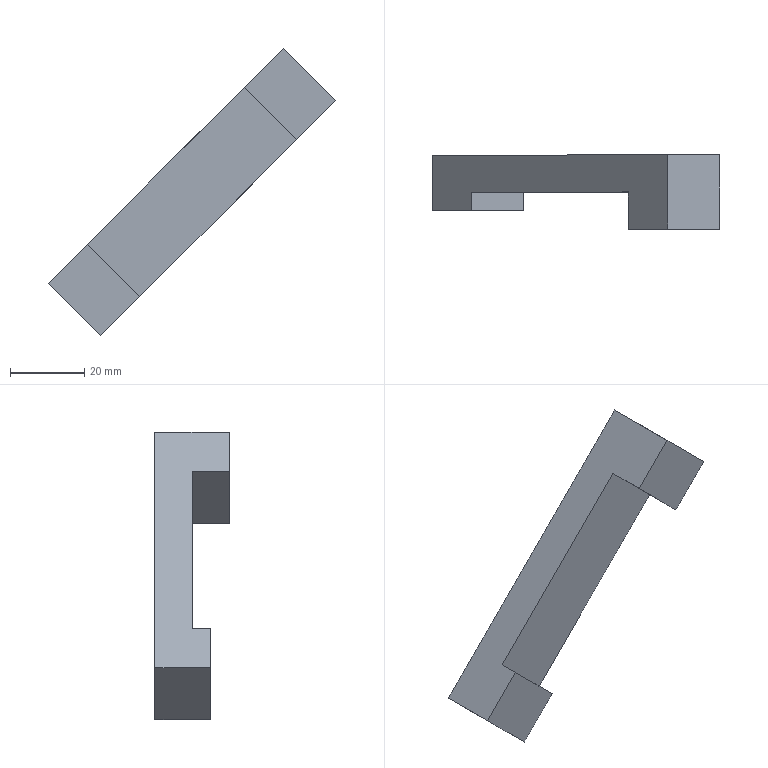Part | NX | features solid 2 | 1 solid | 10 faces | box 77.441 x 20 x 77.441 mm | volume 22280 mm3 | plane 10
STEP:
#1=CARTESIAN_POINT('',(973.987,320.,-96.61));
#2=VERTEX_POINT('',#1);
#3=CARTESIAN_POINT('',(988.034,320.,-110.657));
#4=VERTEX_POINT('',#3);
#5=CARTESIAN_POINT('',(975.003,320.,-97.625));
#6=DIRECTION('',(0.7071,0.,-0.7071));
#7=VECTOR('',#6,1000.);
#8=LINE('',#5,#7);
#9=EDGE_CURVE('',#2,#4,#8,.T.);
#10=ORIENTED_EDGE('',*,*,#9,.T.);
#11=CARTESIAN_POINT('',(1030.215,320.,-68.476));
#12=VERTEX_POINT('',#11);
#13=CARTESIAN_POINT('',(1044.239,320.,-54.452));
#14=DIRECTION('',(0.7071,0.,0.7071));
#15=VECTOR('',#14,1000.);
#16=LINE('',#13,#15);
#17=EDGE_CURVE('',#12,#4,#16,.F.);
#18=ORIENTED_EDGE('',*,*,#17,.F.);
#19=CARTESIAN_POINT('',(1016.168,320.,-54.429));
#20=VERTEX_POINT('',#19);
#21=CARTESIAN_POINT('',(1017.184,320.,-55.445));
#22=DIRECTION('',(-0.7071,0.,0.7071));
#23=VECTOR('',#22,1000.);
#24=LINE('',#21,#23);
#25=EDGE_CURVE('',#12,#20,#24,.T.);
#26=ORIENTED_EDGE('',*,*,#25,.T.);
#27=CARTESIAN_POINT('',(1023.864,320.,-46.733));
#28=DIRECTION('',(-0.7071,0.,-0.7071));
#29=VECTOR('',#28,1000.);
#30=LINE('',#27,#29);
#31=EDGE_CURVE('',#20,#2,#30,.T.);
#32=ORIENTED_EDGE('',*,*,#31,.T.);
#33=EDGE_LOOP('',(#10,#18,#26,#32));
#34=FACE_BOUND('',#33,.T.);
#35=CARTESIAN_POINT('',(1031.207,320.,-41.421));
#36=DIRECTION('',(0.,1.,0.));
#37=DIRECTION('',(-0.9796,0.,0.2008));
#38=AXIS2_PLACEMENT_3D('',#35,#36,#37);
#39=PLANE('',#38);
#40=ADVANCED_FACE('',(#34),#39,.F.);
#41=CARTESIAN_POINT('',(988.034,315.,-110.657));
#42=VERTEX_POINT('',#41);
#43=CARTESIAN_POINT('',(988.034,320.,-110.657));
#44=DIRECTION('',(0.,-1.,0.));
#45=VECTOR('',#44,1000.);
#46=LINE('',#43,#45);
#47=EDGE_CURVE('',#42,#4,#46,.F.);
#48=ORIENTED_EDGE('',*,*,#47,.F.);
#49=CARTESIAN_POINT('',(977.428,315.,-121.263));
#50=VERTEX_POINT('',#49);
#51=CARTESIAN_POINT('',(980.599,315.,-118.092));
#52=DIRECTION('',(-0.7071,0.,-0.7071));
#53=VECTOR('',#52,1000.);
#54=LINE('',#51,#53);
#55=EDGE_CURVE('',#50,#42,#54,.F.);
#56=ORIENTED_EDGE('',*,*,#55,.F.);
#57=CARTESIAN_POINT('',(977.428,330.,-121.263));
#58=VERTEX_POINT('',#57);
#59=CARTESIAN_POINT('',(977.428,320.,-121.263));
#60=DIRECTION('',(0.,-1.,0.));
#61=VECTOR('',#60,1000.);
#62=LINE('',#59,#61);
#63=EDGE_CURVE('',#50,#58,#62,.F.);
#64=ORIENTED_EDGE('',*,*,#63,.T.);
#65=CARTESIAN_POINT('',(1040.822,330.,-57.869));
#66=VERTEX_POINT('',#65);
#67=CARTESIAN_POINT('',(1044.239,330.,-54.452));
#68=DIRECTION('',(0.7071,0.,0.7071));
#69=VECTOR('',#68,1000.);
#70=LINE('',#67,#69);
#71=EDGE_CURVE('',#66,#58,#70,.F.);
#72=ORIENTED_EDGE('',*,*,#71,.F.);
#73=CARTESIAN_POINT('',(1040.822,310.,-57.869));
#74=VERTEX_POINT('',#73);
#75=CARTESIAN_POINT('',(1040.822,320.,-57.869));
#76=DIRECTION('',(0.,1.,0.));
#77=VECTOR('',#76,1000.);
#78=LINE('',#75,#77);
#79=EDGE_CURVE('',#66,#74,#78,.F.);
#80=ORIENTED_EDGE('',*,*,#79,.T.);
#81=CARTESIAN_POINT('',(1030.215,310.,-68.476));
#82=VERTEX_POINT('',#81);
#83=CARTESIAN_POINT('',(1044.239,310.,-54.452));
#84=DIRECTION('',(0.7071,0.,0.7071));
#85=VECTOR('',#84,1000.);
#86=LINE('',#83,#85);
#87=EDGE_CURVE('',#74,#82,#86,.F.);
#88=ORIENTED_EDGE('',*,*,#87,.T.);
#89=CARTESIAN_POINT('',(1030.215,320.,-68.476));
#90=DIRECTION('',(0.,1.,0.));
#91=VECTOR('',#90,1000.);
#92=LINE('',#89,#91);
#93=EDGE_CURVE('',#12,#82,#92,.F.);
#94=ORIENTED_EDGE('',*,*,#93,.F.);
#95=ORIENTED_EDGE('',*,*,#17,.T.);
#96=EDGE_LOOP('',(#48,#56,#64,#72,#80,#88,#94,#95));
#97=FACE_BOUND('',#96,.T.);
#98=CARTESIAN_POINT('',(1036.273,320.,-62.418));
#99=DIRECTION('',(0.7071,0.,-0.7071));
#100=DIRECTION('',(-0.7071,0.,-0.7071));
#101=AXIS2_PLACEMENT_3D('',#98,#99,#100);
#102=PLANE('',#101);
#103=ADVANCED_FACE('',(#97),#102,.T.);
#104=CARTESIAN_POINT('',(963.381,330.,-107.216));
#105=VERTEX_POINT('',#104);
#106=CARTESIAN_POINT('',(963.381,315.,-107.216));
#107=VERTEX_POINT('',#106);
#108=CARTESIAN_POINT('',(963.381,320.,-107.216));
#109=DIRECTION('',(0.,-1.,0.));
#110=VECTOR('',#109,1000.);
#111=LINE('',#108,#110);
#112=EDGE_CURVE('',#105,#107,#111,.T.);
#113=ORIENTED_EDGE('',*,*,#112,.T.);
#114=CARTESIAN_POINT('',(973.987,315.,-96.61));
#115=VERTEX_POINT('',#114);
#116=CARTESIAN_POINT('',(1023.864,315.,-46.733));
#117=DIRECTION('',(0.7071,0.,0.7071));
#118=VECTOR('',#117,1000.);
#119=LINE('',#116,#118);
#120=EDGE_CURVE('',#107,#115,#119,.T.);
#121=ORIENTED_EDGE('',*,*,#120,.T.);
#122=CARTESIAN_POINT('',(973.987,320.,-96.61));
#123=DIRECTION('',(0.,-1.,0.));
#124=VECTOR('',#123,1000.);
#125=LINE('',#122,#124);
#126=EDGE_CURVE('',#2,#115,#125,.T.);
#127=ORIENTED_EDGE('',*,*,#126,.F.);
#128=ORIENTED_EDGE('',*,*,#31,.F.);
#129=CARTESIAN_POINT('',(1016.168,310.,-54.429));
#130=VERTEX_POINT('',#129);
#131=CARTESIAN_POINT('',(1016.168,320.,-54.429));
#132=DIRECTION('',(0.,1.,0.));
#133=VECTOR('',#132,1000.);
#134=LINE('',#131,#133);
#135=EDGE_CURVE('',#130,#20,#134,.T.);
#136=ORIENTED_EDGE('',*,*,#135,.F.);
#137=CARTESIAN_POINT('',(1026.775,310.,-43.822));
#138=VERTEX_POINT('',#137);
#139=CARTESIAN_POINT('',(1023.864,310.,-46.733));
#140=DIRECTION('',(-0.7071,0.,-0.7071));
#141=VECTOR('',#140,1000.);
#142=LINE('',#139,#141);
#143=EDGE_CURVE('',#138,#130,#142,.T.);
#144=ORIENTED_EDGE('',*,*,#143,.F.);
#145=CARTESIAN_POINT('',(1026.775,330.,-43.822));
#146=VERTEX_POINT('',#145);
#147=CARTESIAN_POINT('',(1026.775,320.,-43.822));
#148=DIRECTION('',(0.,1.,0.));
#149=VECTOR('',#148,1000.);
#150=LINE('',#147,#149);
#151=EDGE_CURVE('',#138,#146,#150,.T.);
#152=ORIENTED_EDGE('',*,*,#151,.T.);
#153=CARTESIAN_POINT('',(1023.864,330.,-46.733));
#154=DIRECTION('',(-0.7071,0.,-0.7071));
#155=VECTOR('',#154,1000.);
#156=LINE('',#153,#155);
#157=EDGE_CURVE('',#146,#105,#156,.T.);
#158=ORIENTED_EDGE('',*,*,#157,.T.);
#159=EDGE_LOOP('',(#113,#121,#127,#128,#136,#144,#152,#158));
#160=FACE_BOUND('',#159,.T.);
#161=CARTESIAN_POINT('',(1023.864,320.,-46.733));
#162=DIRECTION('',(0.7071,0.,-0.7071));
#163=DIRECTION('',(-0.7071,0.,-0.7071));
#164=AXIS2_PLACEMENT_3D('',#161,#162,#163);
#165=PLANE('',#164);
#166=ADVANCED_FACE('',(#160),#165,.F.);
#167=CARTESIAN_POINT('',(964.397,330.,-108.232));
#168=DIRECTION('',(0.7071,0.,-0.7071));
#169=VECTOR('',#168,1000.);
#170=LINE('',#167,#169);
#171=EDGE_CURVE('',#105,#58,#170,.T.);
#172=ORIENTED_EDGE('',*,*,#171,.F.);
#173=ORIENTED_EDGE('',*,*,#157,.F.);
#174=CARTESIAN_POINT('',(1027.79,330.,-44.838));
#175=DIRECTION('',(-0.7071,0.,0.7071));
#176=VECTOR('',#175,1000.);
#177=LINE('',#174,#176);
#178=EDGE_CURVE('',#66,#146,#177,.T.);
#179=ORIENTED_EDGE('',*,*,#178,.F.);
#180=ORIENTED_EDGE('',*,*,#71,.T.);
#181=EDGE_LOOP('',(#172,#173,#179,#180));
#182=FACE_BOUND('',#181,.T.);
#183=CARTESIAN_POINT('',(1031.207,330.,-41.421));
#184=DIRECTION('',(0.,1.,0.));
#185=DIRECTION('',(-0.9796,0.,0.2008));
#186=AXIS2_PLACEMENT_3D('',#183,#184,#185);
#187=PLANE('',#186);
#188=ADVANCED_FACE('',(#182),#187,.T.);
#189=CARTESIAN_POINT('',(1027.79,310.,-44.838));
#190=DIRECTION('',(-0.7071,0.,0.7071));
#191=VECTOR('',#190,1000.);
#192=LINE('',#189,#191);
#193=EDGE_CURVE('',#74,#138,#192,.T.);
#194=ORIENTED_EDGE('',*,*,#193,.T.);
#195=ORIENTED_EDGE('',*,*,#143,.T.);
#196=CARTESIAN_POINT('',(1017.184,310.,-55.445));
#197=DIRECTION('',(-0.7071,0.,0.7071));
#198=VECTOR('',#197,1000.);
#199=LINE('',#196,#198);
#200=EDGE_CURVE('',#82,#130,#199,.T.);
#201=ORIENTED_EDGE('',*,*,#200,.F.);
#202=ORIENTED_EDGE('',*,*,#87,.F.);
#203=EDGE_LOOP('',(#194,#195,#201,#202));
#204=FACE_BOUND('',#203,.T.);
#205=CARTESIAN_POINT('',(1031.207,310.,-41.421));
#206=DIRECTION('',(0.,1.,0.));
#207=DIRECTION('',(-0.9796,0.,0.2008));
#208=AXIS2_PLACEMENT_3D('',#205,#206,#207);
#209=PLANE('',#208);
#210=ADVANCED_FACE('',(#204),#209,.F.);
#211=ORIENTED_EDGE('',*,*,#55,.T.);
#212=CARTESIAN_POINT('',(975.003,315.,-97.625));
#213=DIRECTION('',(-0.7071,0.,0.7071));
#214=VECTOR('',#213,1000.);
#215=LINE('',#212,#214);
#216=EDGE_CURVE('',#42,#115,#215,.T.);
#217=ORIENTED_EDGE('',*,*,#216,.T.);
#218=ORIENTED_EDGE('',*,*,#120,.F.);
#219=CARTESIAN_POINT('',(964.397,315.,-108.232));
#220=DIRECTION('',(-0.7071,0.,0.7071));
#221=VECTOR('',#220,1000.);
#222=LINE('',#219,#221);
#223=EDGE_CURVE('',#50,#107,#222,.T.);
#224=ORIENTED_EDGE('',*,*,#223,.F.);
#225=EDGE_LOOP('',(#211,#217,#218,#224));
#226=FACE_BOUND('',#225,.T.);
#227=CARTESIAN_POINT('',(967.568,315.,-105.06));
#228=DIRECTION('',(0.,-1.,0.));
#229=DIRECTION('',(0.9796,0.,-0.2008));
#230=AXIS2_PLACEMENT_3D('',#227,#228,#229);
#231=PLANE('',#230);
#232=ADVANCED_FACE('',(#226),#231,.T.);
#233=ORIENTED_EDGE('',*,*,#171,.T.);
#234=ORIENTED_EDGE('',*,*,#63,.F.);
#235=ORIENTED_EDGE('',*,*,#223,.T.);
#236=ORIENTED_EDGE('',*,*,#112,.F.);
#237=EDGE_LOOP('',(#233,#234,#235,#236));
#238=FACE_BOUND('',#237,.T.);
#239=CARTESIAN_POINT('',(993.082,180.,-136.918));
#240=DIRECTION('',(-0.7071,0.,-0.7071));
#241=DIRECTION('',(0.7071,0.,-0.7071));
#242=AXIS2_PLACEMENT_3D('',#239,#240,#241);
#243=PLANE('',#242);
#244=ADVANCED_FACE('',(#238),#243,.T.);
#245=ORIENTED_EDGE('',*,*,#178,.T.);
#246=ORIENTED_EDGE('',*,*,#151,.F.);
#247=ORIENTED_EDGE('',*,*,#193,.F.);
#248=ORIENTED_EDGE('',*,*,#79,.F.);
#249=EDGE_LOOP('',(#245,#246,#247,#248));
#250=FACE_BOUND('',#249,.T.);
#251=CARTESIAN_POINT('',(1029.012,320.,-46.059));
#252=DIRECTION('',(0.7071,0.,0.7071));
#253=DIRECTION('',(-0.7071,0.,0.7071));
#254=AXIS2_PLACEMENT_3D('',#251,#252,#253);
#255=PLANE('',#254);
#256=ADVANCED_FACE('',(#250),#255,.T.);
#257=ORIENTED_EDGE('',*,*,#93,.T.);
#258=ORIENTED_EDGE('',*,*,#200,.T.);
#259=ORIENTED_EDGE('',*,*,#135,.T.);
#260=ORIENTED_EDGE('',*,*,#25,.F.);
#261=EDGE_LOOP('',(#257,#258,#259,#260));
#262=FACE_BOUND('',#261,.T.);
#263=CARTESIAN_POINT('',(1018.405,320.,-56.666));
#264=DIRECTION('',(0.7071,0.,0.7071));
#265=DIRECTION('',(-0.7071,0.,0.7071));
#266=AXIS2_PLACEMENT_3D('',#263,#264,#265);
#267=PLANE('',#266);
#268=ADVANCED_FACE('',(#262),#267,.F.);
#269=ORIENTED_EDGE('',*,*,#126,.T.);
#270=ORIENTED_EDGE('',*,*,#216,.F.);
#271=ORIENTED_EDGE('',*,*,#47,.T.);
#272=ORIENTED_EDGE('',*,*,#9,.F.);
#273=EDGE_LOOP('',(#269,#270,#271,#272));
#274=FACE_BOUND('',#273,.T.);
#275=CARTESIAN_POINT('',(1003.689,180.,-126.311));
#276=DIRECTION('',(-0.7071,0.,-0.7071));
#277=DIRECTION('',(0.7071,0.,-0.7071));
#278=AXIS2_PLACEMENT_3D('',#275,#276,#277);
#279=PLANE('',#278);
#280=ADVANCED_FACE('',(#274),#279,.F.);
#281=CLOSED_SHELL('',(#40,#103,#166,#188,#210,#232,#244,#256,#268,#280));
#282=MANIFOLD_SOLID_BREP('',#281);
#283=(LENGTH_UNIT()NAMED_UNIT(*)SI_UNIT(.MILLI.,.METRE.));
#284=UNCERTAINTY_MEASURE_WITH_UNIT(LENGTH_MEASURE(0.00001),#283,'','');
#285=(NAMED_UNIT(*)PLANE_ANGLE_UNIT()SI_UNIT($,.RADIAN.));
#286=(NAMED_UNIT(*)SI_UNIT($,.STERADIAN.)SOLID_ANGLE_UNIT());
#287=(GEOMETRIC_REPRESENTATION_CONTEXT(3)GLOBAL_UNCERTAINTY_ASSIGNED_CONTEXT((#284))GLOBAL_UNIT_ASSIGNED_CONTEXT((#283,#285,#286))REPRESENTATION_CONTEXT('',''));
#288=ADVANCED_BREP_SHAPE_REPRESENTATION('',(#282),#287);